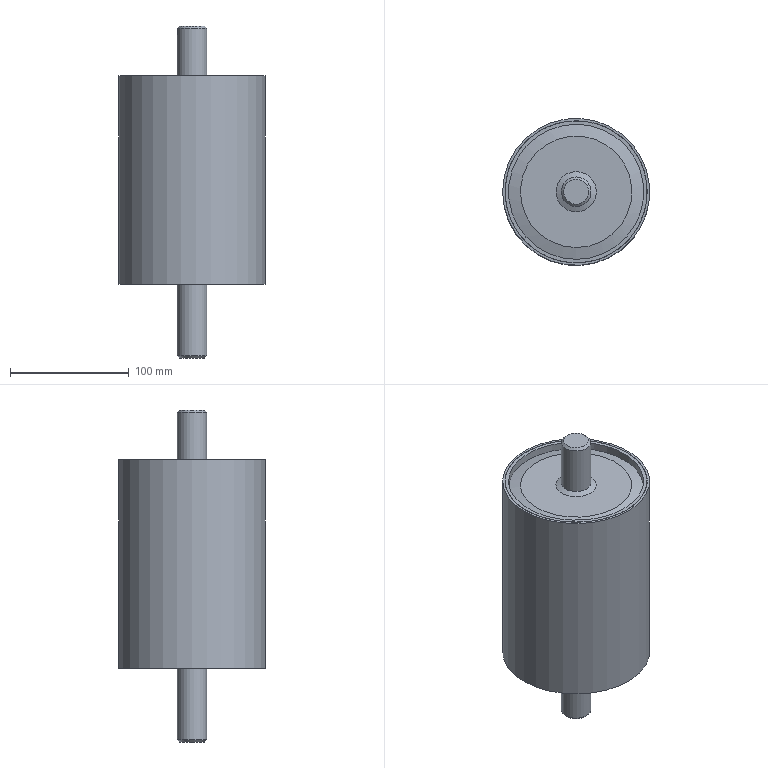Part | STEP file | Pulley | 2 solids | 29 faces | box 124 x 124 x 280 mm | volume 525359 mm3 | cone 10 | plane 10 | cylinder 9 | commonest cylinder face diameters 25 x3 114 x3 120 x2 124 x1
STEP:
#1=CARTESIAN_POINT('',(0.,-10.5,-150.));
#2=VERTEX_POINT('',#1);
#3=CARTESIAN_POINT('',(0.,0.,-150.));
#4=DIRECTION('',(0.,0.,1.));
#5=DIRECTION('',(0.,1.,0.));
#6=AXIS2_PLACEMENT_3D('',#3,#4,#5);
#7=CIRCLE('',#6,10.5);
#8=EDGE_CURVE('',#2,#2,#7,.T.);
#9=ORIENTED_EDGE('',*,*,#8,.T.);
#10=CARTESIAN_POINT('',(0.,-12.5,-148.));
#11=VERTEX_POINT('',#10);
#12=CARTESIAN_POINT('',(0.,-11.5,-149.));
#13=DIRECTION('',(0.,-0.7071,0.7071));
#14=VECTOR('',#13,11.5);
#15=LINE('',#12,#14);
#16=EDGE_CURVE('',#2,#11,#15,.T.);
#17=ORIENTED_EDGE('',*,*,#16,.T.);
#18=CARTESIAN_POINT('',(0.,0.,-148.));
#19=DIRECTION('',(0.,0.,-1.));
#20=DIRECTION('',(0.,1.,0.));
#21=AXIS2_PLACEMENT_3D('',#18,#19,#20);
#22=CIRCLE('',#21,12.5);
#23=EDGE_CURVE('',#11,#11,#22,.T.);
#24=ORIENTED_EDGE('',*,*,#23,.T.);
#25=ORIENTED_EDGE('',*,*,#16,.F.);
#26=EDGE_LOOP('',(#9,#17,#24,#25));
#27=FACE_OUTER_BOUND('',#26,.T.);
#28=CARTESIAN_POINT('',(0.,0.,-149.));
#29=DIRECTION('',(0.,0.,1.));
#30=DIRECTION('',(0.,1.,0.));
#31=AXIS2_PLACEMENT_3D('',#28,#29,#30);
#32=CONICAL_SURFACE('',#31,11.5,0.7854);
#33=ADVANCED_FACE('',(#27),#32,.T.);
#34=ORIENTED_EDGE('',*,*,#8,.F.);
#35=EDGE_LOOP('',(#34));
#36=FACE_OUTER_BOUND('',#35,.T.);
#37=CARTESIAN_POINT('',(0.,0.,-150.));
#38=DIRECTION('',(0.,0.,-1.));
#39=DIRECTION('',(-1.,0.,0.));
#40=AXIS2_PLACEMENT_3D('',#37,#38,#39);
#41=PLANE('',#40);
#42=ADVANCED_FACE('',(#36),#41,.T.);
#43=ORIENTED_EDGE('',*,*,#23,.F.);
#44=CARTESIAN_POINT('',(0.,-12.5,-86.098));
#45=VERTEX_POINT('',#44);
#46=CARTESIAN_POINT('',(0.,-12.5,-108.049));
#47=DIRECTION('',(0.,0.,1.));
#48=VECTOR('',#47,12.5);
#49=LINE('',#46,#48);
#50=EDGE_CURVE('',#11,#45,#49,.T.);
#51=ORIENTED_EDGE('',*,*,#50,.T.);
#52=CARTESIAN_POINT('',(0.,0.,-86.098));
#53=DIRECTION('',(0.,0.,-1.));
#54=DIRECTION('',(1.,0.,0.));
#55=AXIS2_PLACEMENT_3D('',#52,#53,#54);
#56=CIRCLE('',#55,12.5);
#57=EDGE_CURVE('',#45,#45,#56,.T.);
#58=ORIENTED_EDGE('',*,*,#57,.T.);
#59=ORIENTED_EDGE('',*,*,#50,.F.);
#60=EDGE_LOOP('',(#43,#51,#58,#59));
#61=FACE_OUTER_BOUND('',#60,.T.);
#62=CARTESIAN_POINT('',(0.,0.,-108.049));
#63=DIRECTION('',(0.,0.,-1.));
#64=DIRECTION('',(0.,1.,0.));
#65=AXIS2_PLACEMENT_3D('',#62,#63,#64);
#66=CYLINDRICAL_SURFACE('',#65,12.5);
#67=ADVANCED_FACE('',(#61),#66,.T.);
#68=CARTESIAN_POINT('',(0.,12.5,128.));
#69=VERTEX_POINT('',#68);
#70=CARTESIAN_POINT('',(0.,-12.5,128.));
#71=VERTEX_POINT('',#70);
#72=CARTESIAN_POINT('',(0.,0.,128.));
#73=DIRECTION('',(0.,0.,1.));
#74=DIRECTION('',(0.,-1.,0.));
#75=AXIS2_PLACEMENT_3D('',#72,#73,#74);
#76=CIRCLE('',#75,12.5);
#77=EDGE_CURVE('',#69,#71,#76,.T.);
#78=ORIENTED_EDGE('',*,*,#77,.T.);
#79=CARTESIAN_POINT('',(0.,0.,128.));
#80=DIRECTION('',(0.,0.,1.));
#81=DIRECTION('',(0.,-1.,0.));
#82=AXIS2_PLACEMENT_3D('',#79,#80,#81);
#83=CIRCLE('',#82,12.5);
#84=EDGE_CURVE('',#71,#69,#83,.T.);
#85=ORIENTED_EDGE('',*,*,#84,.T.);
#86=CARTESIAN_POINT('',(0.,10.5,130.));
#87=VERTEX_POINT('',#86);
#88=CARTESIAN_POINT('',(0.,11.5,129.));
#89=DIRECTION('',(0.,-0.7071,0.7071));
#90=VECTOR('',#89,11.5);
#91=LINE('',#88,#90);
#92=EDGE_CURVE('',#69,#87,#91,.T.);
#93=ORIENTED_EDGE('',*,*,#92,.T.);
#94=CARTESIAN_POINT('',(0.,0.,130.));
#95=DIRECTION('',(0.,0.,-1.));
#96=DIRECTION('',(0.,-1.,0.));
#97=AXIS2_PLACEMENT_3D('',#94,#95,#96);
#98=CIRCLE('',#97,10.5);
#99=EDGE_CURVE('',#87,#87,#98,.T.);
#100=ORIENTED_EDGE('',*,*,#99,.T.);
#101=ORIENTED_EDGE('',*,*,#92,.F.);
#102=EDGE_LOOP('',(#78,#85,#93,#100,#101));
#103=FACE_OUTER_BOUND('',#102,.T.);
#104=CARTESIAN_POINT('',(0.,0.,129.));
#105=DIRECTION('',(0.,0.,-1.));
#106=DIRECTION('',(0.,-1.,0.));
#107=AXIS2_PLACEMENT_3D('',#104,#105,#106);
#108=CONICAL_SURFACE('',#107,11.5,0.7854);
#109=ADVANCED_FACE('',(#103),#108,.T.);
#110=ORIENTED_EDGE('',*,*,#99,.F.);
#111=EDGE_LOOP('',(#110));
#112=FACE_OUTER_BOUND('',#111,.T.);
#113=CARTESIAN_POINT('',(0.,12.5,130.));
#114=DIRECTION('',(0.,0.,1.));
#115=DIRECTION('',(1.,0.,0.));
#116=AXIS2_PLACEMENT_3D('',#113,#114,#115);
#117=PLANE('',#116);
#118=ADVANCED_FACE('',(#112),#117,.T.);
#119=CARTESIAN_POINT('',(0.,-12.5,86.098));
#120=VERTEX_POINT('',#119);
#121=CARTESIAN_POINT('',(0.,0.,86.098));
#122=DIRECTION('',(0.,0.,-1.));
#123=DIRECTION('',(1.,0.,0.));
#124=AXIS2_PLACEMENT_3D('',#121,#122,#123);
#125=CIRCLE('',#124,12.5);
#126=EDGE_CURVE('',#120,#120,#125,.T.);
#127=ORIENTED_EDGE('',*,*,#126,.F.);
#128=CARTESIAN_POINT('',(0.,-12.5,108.049));
#129=DIRECTION('',(0.,0.,1.));
#130=VECTOR('',#129,12.5);
#131=LINE('',#128,#130);
#132=EDGE_CURVE('',#120,#71,#131,.T.);
#133=ORIENTED_EDGE('',*,*,#132,.T.);
#134=ORIENTED_EDGE('',*,*,#77,.F.);
#135=ORIENTED_EDGE('',*,*,#84,.F.);
#136=ORIENTED_EDGE('',*,*,#132,.F.);
#137=EDGE_LOOP('',(#127,#133,#134,#135,#136));
#138=FACE_OUTER_BOUND('',#137,.T.);
#139=CARTESIAN_POINT('',(0.,0.,108.049));
#140=DIRECTION('',(0.,0.,-1.));
#141=DIRECTION('',(0.,1.,0.));
#142=AXIS2_PLACEMENT_3D('',#139,#140,#141);
#143=CYLINDRICAL_SURFACE('',#142,12.5);
#144=ADVANCED_FACE('',(#138),#143,.T.);
#145=CARTESIAN_POINT('',(0.,-17.,84.));
#146=VERTEX_POINT('',#145);
#147=CARTESIAN_POINT('',(0.,0.,84.));
#148=DIRECTION('',(0.,0.,-1.));
#149=DIRECTION('',(1.,0.,0.));
#150=AXIS2_PLACEMENT_3D('',#147,#148,#149);
#151=CIRCLE('',#150,17.);
#152=EDGE_CURVE('',#146,#146,#151,.T.);
#153=ORIENTED_EDGE('',*,*,#152,.F.);
#154=CARTESIAN_POINT('',(0.,-14.75,85.049));
#155=DIRECTION('',(0.,0.9063,0.4226));
#156=VECTOR('',#155,14.75);
#157=LINE('',#154,#156);
#158=EDGE_CURVE('',#146,#120,#157,.T.);
#159=ORIENTED_EDGE('',*,*,#158,.T.);
#160=ORIENTED_EDGE('',*,*,#126,.T.);
#161=ORIENTED_EDGE('',*,*,#158,.F.);
#162=EDGE_LOOP('',(#153,#159,#160,#161));
#163=FACE_OUTER_BOUND('',#162,.T.);
#164=CARTESIAN_POINT('',(0.,0.,85.049));
#165=DIRECTION('',(0.,0.,-1.));
#166=DIRECTION('',(0.,1.,0.));
#167=AXIS2_PLACEMENT_3D('',#164,#165,#166);
#168=CONICAL_SURFACE('',#167,14.75,1.134);
#169=ADVANCED_FACE('',(#163),#168,.T.);
#170=CARTESIAN_POINT('',(0.,-47.,84.));
#171=VERTEX_POINT('',#170);
#172=CARTESIAN_POINT('',(0.,0.,84.));
#173=DIRECTION('',(0.,0.,-1.));
#174=DIRECTION('',(1.,0.,0.));
#175=AXIS2_PLACEMENT_3D('',#172,#173,#174);
#176=CIRCLE('',#175,47.);
#177=EDGE_CURVE('',#171,#171,#176,.T.);
#178=ORIENTED_EDGE('',*,*,#177,.F.);
#179=EDGE_LOOP('',(#178));
#180=FACE_OUTER_BOUND('',#179,.T.);
#181=ORIENTED_EDGE('',*,*,#152,.T.);
#182=EDGE_LOOP('',(#181));
#183=FACE_BOUND('',#182,.T.);
#184=CARTESIAN_POINT('',(0.,47.,84.));
#185=DIRECTION('',(0.,0.,1.));
#186=DIRECTION('',(1.,0.,0.));
#187=AXIS2_PLACEMENT_3D('',#184,#185,#186);
#188=PLANE('',#187);
#189=ADVANCED_FACE('',(#180,#183),#188,.T.);
#190=CARTESIAN_POINT('',(0.,-57.,81.321));
#191=VERTEX_POINT('',#190);
#192=CARTESIAN_POINT('',(0.,0.,81.321));
#193=DIRECTION('',(0.,0.,-1.));
#194=DIRECTION('',(1.,0.,0.));
#195=AXIS2_PLACEMENT_3D('',#192,#193,#194);
#196=CIRCLE('',#195,57.);
#197=EDGE_CURVE('',#191,#191,#196,.T.);
#198=ORIENTED_EDGE('',*,*,#197,.F.);
#199=CARTESIAN_POINT('',(0.,-52.,82.66));
#200=DIRECTION('',(0.,0.9659,0.2588));
#201=VECTOR('',#200,52.);
#202=LINE('',#199,#201);
#203=EDGE_CURVE('',#191,#171,#202,.T.);
#204=ORIENTED_EDGE('',*,*,#203,.T.);
#205=ORIENTED_EDGE('',*,*,#177,.T.);
#206=ORIENTED_EDGE('',*,*,#203,.F.);
#207=EDGE_LOOP('',(#198,#204,#205,#206));
#208=FACE_OUTER_BOUND('',#207,.T.);
#209=CARTESIAN_POINT('',(0.,0.,82.66));
#210=DIRECTION('',(0.,0.,-1.));
#211=DIRECTION('',(0.,1.,0.));
#212=AXIS2_PLACEMENT_3D('',#209,#210,#211);
#213=CONICAL_SURFACE('',#212,52.,1.309);
#214=ADVANCED_FACE('',(#208),#213,.T.);
#215=ORIENTED_EDGE('',*,*,#197,.T.);
#216=CARTESIAN_POINT('',(0.,-57.,88.));
#217=VERTEX_POINT('',#216);
#218=CARTESIAN_POINT('',(0.,-57.,84.66));
#219=DIRECTION('',(0.,0.,1.));
#220=VECTOR('',#219,57.);
#221=LINE('',#218,#220);
#222=EDGE_CURVE('',#191,#217,#221,.T.);
#223=ORIENTED_EDGE('',*,*,#222,.T.);
#224=CARTESIAN_POINT('',(0.,0.,88.));
#225=DIRECTION('',(0.,0.,-1.));
#226=DIRECTION('',(1.,0.,0.));
#227=AXIS2_PLACEMENT_3D('',#224,#225,#226);
#228=CIRCLE('',#227,57.);
#229=EDGE_CURVE('',#217,#217,#228,.T.);
#230=ORIENTED_EDGE('',*,*,#229,.F.);
#231=ORIENTED_EDGE('',*,*,#222,.F.);
#232=EDGE_LOOP('',(#215,#223,#230,#231));
#233=FACE_OUTER_BOUND('',#232,.T.);
#234=CARTESIAN_POINT('',(0.,0.,84.66));
#235=DIRECTION('',(0.,0.,-1.));
#236=DIRECTION('',(0.,1.,0.));
#237=AXIS2_PLACEMENT_3D('',#234,#235,#236);
#238=CYLINDRICAL_SURFACE('',#237,57.);
#239=ADVANCED_FACE('',(#233),#238,.F.);
#240=CARTESIAN_POINT('',(0.,-60.,88.));
#241=VERTEX_POINT('',#240);
#242=CARTESIAN_POINT('',(0.,0.,88.));
#243=DIRECTION('',(0.,0.,-1.));
#244=DIRECTION('',(1.,0.,0.));
#245=AXIS2_PLACEMENT_3D('',#242,#243,#244);
#246=CIRCLE('',#245,60.);
#247=EDGE_CURVE('',#241,#241,#246,.T.);
#248=ORIENTED_EDGE('',*,*,#247,.F.);
#249=EDGE_LOOP('',(#248));
#250=FACE_OUTER_BOUND('',#249,.T.);
#251=ORIENTED_EDGE('',*,*,#229,.T.);
#252=EDGE_LOOP('',(#251));
#253=FACE_BOUND('',#252,.T.);
#254=CARTESIAN_POINT('',(0.,60.,88.));
#255=DIRECTION('',(0.,0.,1.));
#256=DIRECTION('',(1.,0.,0.));
#257=AXIS2_PLACEMENT_3D('',#254,#255,#256);
#258=PLANE('',#257);
#259=ADVANCED_FACE('',(#250,#253),#258,.T.);
#260=CARTESIAN_POINT('',(0.,-60.,-88.));
#261=VERTEX_POINT('',#260);
#262=CARTESIAN_POINT('',(0.,0.,-88.));
#263=DIRECTION('',(0.,0.,-1.));
#264=DIRECTION('',(1.,0.,0.));
#265=AXIS2_PLACEMENT_3D('',#262,#263,#264);
#266=CIRCLE('',#265,60.);
#267=EDGE_CURVE('',#261,#261,#266,.T.);
#268=ORIENTED_EDGE('',*,*,#267,.F.);
#269=CARTESIAN_POINT('',(0.,-60.,0.));
#270=DIRECTION('',(0.,0.,1.));
#271=VECTOR('',#270,60.);
#272=LINE('',#269,#271);
#273=EDGE_CURVE('',#261,#241,#272,.T.);
#274=ORIENTED_EDGE('',*,*,#273,.T.);
#275=ORIENTED_EDGE('',*,*,#247,.T.);
#276=ORIENTED_EDGE('',*,*,#273,.F.);
#277=EDGE_LOOP('',(#268,#274,#275,#276));
#278=FACE_OUTER_BOUND('',#277,.T.);
#279=CARTESIAN_POINT('',(0.,0.,0.));
#280=DIRECTION('',(0.,0.,-1.));
#281=DIRECTION('',(0.,1.,0.));
#282=AXIS2_PLACEMENT_3D('',#279,#280,#281);
#283=CYLINDRICAL_SURFACE('',#282,60.);
#284=ADVANCED_FACE('',(#278),#283,.T.);
#285=ORIENTED_EDGE('',*,*,#267,.T.);
#286=EDGE_LOOP('',(#285));
#287=FACE_OUTER_BOUND('',#286,.T.);
#288=CARTESIAN_POINT('',(0.,-57.,-88.));
#289=VERTEX_POINT('',#288);
#290=CARTESIAN_POINT('',(0.,0.,-88.));
#291=DIRECTION('',(0.,0.,-1.));
#292=DIRECTION('',(1.,0.,0.));
#293=AXIS2_PLACEMENT_3D('',#290,#291,#292);
#294=CIRCLE('',#293,57.);
#295=EDGE_CURVE('',#289,#289,#294,.T.);
#296=ORIENTED_EDGE('',*,*,#295,.F.);
#297=EDGE_LOOP('',(#296));
#298=FACE_BOUND('',#297,.T.);
#299=CARTESIAN_POINT('',(0.,57.,-88.));
#300=DIRECTION('',(0.,0.,-1.));
#301=DIRECTION('',(-1.,0.,0.));
#302=AXIS2_PLACEMENT_3D('',#299,#300,#301);
#303=PLANE('',#302);
#304=ADVANCED_FACE('',(#287,#298),#303,.T.);
#305=ORIENTED_EDGE('',*,*,#295,.T.);
#306=CARTESIAN_POINT('',(0.,-57.,-81.321));
#307=VERTEX_POINT('',#306);
#308=CARTESIAN_POINT('',(0.,-57.,-84.66));
#309=DIRECTION('',(0.,0.,1.));
#310=VECTOR('',#309,57.);
#311=LINE('',#308,#310);
#312=EDGE_CURVE('',#289,#307,#311,.T.);
#313=ORIENTED_EDGE('',*,*,#312,.T.);
#314=CARTESIAN_POINT('',(0.,0.,-81.321));
#315=DIRECTION('',(0.,0.,-1.));
#316=DIRECTION('',(1.,0.,0.));
#317=AXIS2_PLACEMENT_3D('',#314,#315,#316);
#318=CIRCLE('',#317,57.);
#319=EDGE_CURVE('',#307,#307,#318,.T.);
#320=ORIENTED_EDGE('',*,*,#319,.F.);
#321=ORIENTED_EDGE('',*,*,#312,.F.);
#322=EDGE_LOOP('',(#305,#313,#320,#321));
#323=FACE_OUTER_BOUND('',#322,.T.);
#324=CARTESIAN_POINT('',(0.,0.,-84.66));
#325=DIRECTION('',(0.,0.,-1.));
#326=DIRECTION('',(0.,1.,0.));
#327=AXIS2_PLACEMENT_3D('',#324,#325,#326);
#328=CYLINDRICAL_SURFACE('',#327,57.);
#329=ADVANCED_FACE('',(#323),#328,.F.);
#330=CARTESIAN_POINT('',(0.,-47.,-84.));
#331=VERTEX_POINT('',#330);
#332=CARTESIAN_POINT('',(0.,0.,-84.));
#333=DIRECTION('',(0.,0.,-1.));
#334=DIRECTION('',(1.,0.,0.));
#335=AXIS2_PLACEMENT_3D('',#332,#333,#334);
#336=CIRCLE('',#335,47.);
#337=EDGE_CURVE('',#331,#331,#336,.T.);
#338=ORIENTED_EDGE('',*,*,#337,.F.);
#339=CARTESIAN_POINT('',(0.,-52.,-82.66));
#340=DIRECTION('',(0.,-0.9659,0.2588));
#341=VECTOR('',#340,52.);
#342=LINE('',#339,#341);
#343=EDGE_CURVE('',#331,#307,#342,.T.);
#344=ORIENTED_EDGE('',*,*,#343,.T.);
#345=ORIENTED_EDGE('',*,*,#319,.T.);
#346=ORIENTED_EDGE('',*,*,#343,.F.);
#347=EDGE_LOOP('',(#338,#344,#345,#346));
#348=FACE_OUTER_BOUND('',#347,.T.);
#349=CARTESIAN_POINT('',(0.,0.,-82.66));
#350=DIRECTION('',(0.,0.,1.));
#351=DIRECTION('',(0.,1.,0.));
#352=AXIS2_PLACEMENT_3D('',#349,#350,#351);
#353=CONICAL_SURFACE('',#352,52.,1.309);
#354=ADVANCED_FACE('',(#348),#353,.T.);
#355=ORIENTED_EDGE('',*,*,#337,.T.);
#356=EDGE_LOOP('',(#355));
#357=FACE_OUTER_BOUND('',#356,.T.);
#358=CARTESIAN_POINT('',(0.,-17.,-84.));
#359=VERTEX_POINT('',#358);
#360=CARTESIAN_POINT('',(0.,0.,-84.));
#361=DIRECTION('',(0.,0.,-1.));
#362=DIRECTION('',(1.,0.,0.));
#363=AXIS2_PLACEMENT_3D('',#360,#361,#362);
#364=CIRCLE('',#363,17.);
#365=EDGE_CURVE('',#359,#359,#364,.T.);
#366=ORIENTED_EDGE('',*,*,#365,.F.);
#367=EDGE_LOOP('',(#366));
#368=FACE_BOUND('',#367,.T.);
#369=CARTESIAN_POINT('',(0.,17.,-84.));
#370=DIRECTION('',(0.,0.,-1.));
#371=DIRECTION('',(-1.,0.,0.));
#372=AXIS2_PLACEMENT_3D('',#369,#370,#371);
#373=PLANE('',#372);
#374=ADVANCED_FACE('',(#357,#368),#373,.T.);
#375=ORIENTED_EDGE('',*,*,#57,.F.);
#376=CARTESIAN_POINT('',(0.,-14.75,-85.049));
#377=DIRECTION('',(0.,-0.9063,0.4226));
#378=VECTOR('',#377,14.75);
#379=LINE('',#376,#378);
#380=EDGE_CURVE('',#45,#359,#379,.T.);
#381=ORIENTED_EDGE('',*,*,#380,.T.);
#382=ORIENTED_EDGE('',*,*,#365,.T.);
#383=ORIENTED_EDGE('',*,*,#380,.F.);
#384=EDGE_LOOP('',(#375,#381,#382,#383));
#385=FACE_OUTER_BOUND('',#384,.T.);
#386=CARTESIAN_POINT('',(0.,0.,-85.049));
#387=DIRECTION('',(0.,0.,1.));
#388=DIRECTION('',(0.,1.,0.));
#389=AXIS2_PLACEMENT_3D('',#386,#387,#388);
#390=CONICAL_SURFACE('',#389,14.75,1.134);
#391=ADVANCED_FACE('',(#385),#390,.T.);
#392=CLOSED_SHELL('',(#33,#42,#67,#109,#118,#144,#169,#189,#214,#239,#259,#284,#304,#329,#354,#374,#391));
#393=CARTESIAN_POINT('',(0.,-12.5,-82.792));
#394=VERTEX_POINT('',#393);
#395=CARTESIAN_POINT('',(0.,0.,-82.792));
#396=DIRECTION('',(0.,0.,-1.));
#397=DIRECTION('',(1.,0.,0.));
#398=AXIS2_PLACEMENT_3D('',#395,#396,#397);
#399=CIRCLE('',#398,12.5);
#400=EDGE_CURVE('',#394,#394,#399,.T.);
#401=ORIENTED_EDGE('',*,*,#400,.T.);
#402=CARTESIAN_POINT('',(0.,-16.335,-81.));
#403=VERTEX_POINT('',#402);
#404=CARTESIAN_POINT('',(0.,-14.417,-81.896));
#405=DIRECTION('',(0.,-0.906,0.4233));
#406=VECTOR('',#405,14.417);
#407=LINE('',#404,#406);
#408=EDGE_CURVE('',#394,#403,#407,.T.);
#409=ORIENTED_EDGE('',*,*,#408,.T.);
#410=CARTESIAN_POINT('',(0.,0.,-81.));
#411=DIRECTION('',(0.,0.,-1.));
#412=DIRECTION('',(1.,0.,0.));
#413=AXIS2_PLACEMENT_3D('',#410,#411,#412);
#414=CIRCLE('',#413,16.335);
#415=EDGE_CURVE('',#403,#403,#414,.T.);
#416=ORIENTED_EDGE('',*,*,#415,.F.);
#417=ORIENTED_EDGE('',*,*,#408,.F.);
#418=EDGE_LOOP('',(#401,#409,#416,#417));
#419=FACE_OUTER_BOUND('',#418,.T.);
#420=CARTESIAN_POINT('',(0.,0.,-81.896));
#421=DIRECTION('',(0.,0.,1.));
#422=DIRECTION('',(0.,1.,0.));
#423=AXIS2_PLACEMENT_3D('',#420,#421,#422);
#424=CONICAL_SURFACE('',#423,14.417,1.134);
#425=ADVANCED_FACE('',(#419),#424,.F.);
#426=ORIENTED_EDGE('',*,*,#400,.F.);
#427=CARTESIAN_POINT('',(0.,-12.5,82.792));
#428=VERTEX_POINT('',#427);
#429=CARTESIAN_POINT('',(0.,-12.5,0.));
#430=DIRECTION('',(0.,0.,1.));
#431=VECTOR('',#430,12.5);
#432=LINE('',#429,#431);
#433=EDGE_CURVE('',#394,#428,#432,.T.);
#434=ORIENTED_EDGE('',*,*,#433,.T.);
#435=CARTESIAN_POINT('',(0.,0.,82.792));
#436=DIRECTION('',(0.,0.,-1.));
#437=DIRECTION('',(1.,0.,0.));
#438=AXIS2_PLACEMENT_3D('',#435,#436,#437);
#439=CIRCLE('',#438,12.5);
#440=EDGE_CURVE('',#428,#428,#439,.T.);
#441=ORIENTED_EDGE('',*,*,#440,.T.);
#442=ORIENTED_EDGE('',*,*,#433,.F.);
#443=EDGE_LOOP('',(#426,#434,#441,#442));
#444=FACE_OUTER_BOUND('',#443,.T.);
#445=CARTESIAN_POINT('',(0.,0.,0.));
#446=DIRECTION('',(0.,0.,-1.));
#447=DIRECTION('',(0.,1.,0.));
#448=AXIS2_PLACEMENT_3D('',#445,#446,#447);
#449=CYLINDRICAL_SURFACE('',#448,12.5);
#450=ADVANCED_FACE('',(#444),#449,.T.);
#451=CARTESIAN_POINT('',(0.,-46.605,-81.));
#452=VERTEX_POINT('',#451);
#453=CARTESIAN_POINT('',(0.,0.,-81.));
#454=DIRECTION('',(0.,0.,-1.));
#455=DIRECTION('',(1.,0.,0.));
#456=AXIS2_PLACEMENT_3D('',#453,#454,#455);
#457=CIRCLE('',#456,46.605);
#458=EDGE_CURVE('',#452,#452,#457,.T.);
#459=ORIENTED_EDGE('',*,*,#458,.F.);
#460=EDGE_LOOP('',(#459));
#461=FACE_OUTER_BOUND('',#460,.T.);
#462=ORIENTED_EDGE('',*,*,#415,.T.);
#463=EDGE_LOOP('',(#462));
#464=FACE_BOUND('',#463,.T.);
#465=CARTESIAN_POINT('',(0.,46.605,-81.));
#466=DIRECTION('',(0.,0.,1.));
#467=DIRECTION('',(1.,0.,0.));
#468=AXIS2_PLACEMENT_3D('',#465,#466,#467);
#469=PLANE('',#468);
#470=ADVANCED_FACE('',(#461,#464),#469,.T.);
#471=CARTESIAN_POINT('',(0.,-16.335,81.));
#472=VERTEX_POINT('',#471);
#473=CARTESIAN_POINT('',(0.,0.,81.));
#474=DIRECTION('',(0.,0.,-1.));
#475=DIRECTION('',(1.,0.,0.));
#476=AXIS2_PLACEMENT_3D('',#473,#474,#475);
#477=CIRCLE('',#476,16.335);
#478=EDGE_CURVE('',#472,#472,#477,.T.);
#479=ORIENTED_EDGE('',*,*,#478,.T.);
#480=CARTESIAN_POINT('',(0.,-14.417,81.896));
#481=DIRECTION('',(0.,0.906,0.4233));
#482=VECTOR('',#481,14.417);
#483=LINE('',#480,#482);
#484=EDGE_CURVE('',#472,#428,#483,.T.);
#485=ORIENTED_EDGE('',*,*,#484,.T.);
#486=ORIENTED_EDGE('',*,*,#440,.F.);
#487=ORIENTED_EDGE('',*,*,#484,.F.);
#488=EDGE_LOOP('',(#479,#485,#486,#487));
#489=FACE_OUTER_BOUND('',#488,.T.);
#490=CARTESIAN_POINT('',(0.,0.,81.896));
#491=DIRECTION('',(0.,0.,-1.));
#492=DIRECTION('',(0.,1.,0.));
#493=AXIS2_PLACEMENT_3D('',#490,#491,#492);
#494=CONICAL_SURFACE('',#493,14.417,1.134);
#495=ADVANCED_FACE('',(#489),#494,.F.);
#496=ORIENTED_EDGE('',*,*,#458,.T.);
#497=CARTESIAN_POINT('',(0.,-57.,-78.218));
#498=VERTEX_POINT('',#497);
#499=CARTESIAN_POINT('',(0.,-51.803,-79.609));
#500=DIRECTION('',(0.,-0.966,0.2585));
#501=VECTOR('',#500,51.803);
#502=LINE('',#499,#501);
#503=EDGE_CURVE('',#452,#498,#502,.T.);
#504=ORIENTED_EDGE('',*,*,#503,.T.);
#505=CARTESIAN_POINT('',(0.,0.,-78.218));
#506=DIRECTION('',(0.,0.,-1.));
#507=DIRECTION('',(1.,0.,0.));
#508=AXIS2_PLACEMENT_3D('',#505,#506,#507);
#509=CIRCLE('',#508,57.);
#510=EDGE_CURVE('',#498,#498,#509,.T.);
#511=ORIENTED_EDGE('',*,*,#510,.F.);
#512=ORIENTED_EDGE('',*,*,#503,.F.);
#513=EDGE_LOOP('',(#496,#504,#511,#512));
#514=FACE_OUTER_BOUND('',#513,.T.);
#515=CARTESIAN_POINT('',(0.,0.,-79.609));
#516=DIRECTION('',(0.,0.,1.));
#517=DIRECTION('',(0.,1.,0.));
#518=AXIS2_PLACEMENT_3D('',#515,#516,#517);
#519=CONICAL_SURFACE('',#518,51.803,1.309);
#520=ADVANCED_FACE('',(#514),#519,.F.);
#521=CARTESIAN_POINT('',(0.,-46.605,81.));
#522=VERTEX_POINT('',#521);
#523=CARTESIAN_POINT('',(0.,0.,81.));
#524=DIRECTION('',(0.,0.,-1.));
#525=DIRECTION('',(1.,0.,0.));
#526=AXIS2_PLACEMENT_3D('',#523,#524,#525);
#527=CIRCLE('',#526,46.605);
#528=EDGE_CURVE('',#522,#522,#527,.T.);
#529=ORIENTED_EDGE('',*,*,#528,.T.);
#530=EDGE_LOOP('',(#529));
#531=FACE_OUTER_BOUND('',#530,.T.);
#532=ORIENTED_EDGE('',*,*,#478,.F.);
#533=EDGE_LOOP('',(#532));
#534=FACE_BOUND('',#533,.T.);
#535=CARTESIAN_POINT('',(0.,16.335,81.));
#536=DIRECTION('',(0.,0.,-1.));
#537=DIRECTION('',(-1.,0.,0.));
#538=AXIS2_PLACEMENT_3D('',#535,#536,#537);
#539=PLANE('',#538);
#540=ADVANCED_FACE('',(#531,#534),#539,.T.);
#541=ORIENTED_EDGE('',*,*,#510,.T.);
#542=CARTESIAN_POINT('',(0.,-57.,78.218));
#543=VERTEX_POINT('',#542);
#544=CARTESIAN_POINT('',(0.,-57.,0.));
#545=DIRECTION('',(0.,0.,1.));
#546=VECTOR('',#545,57.);
#547=LINE('',#544,#546);
#548=EDGE_CURVE('',#498,#543,#547,.T.);
#549=ORIENTED_EDGE('',*,*,#548,.T.);
#550=CARTESIAN_POINT('',(0.,0.,78.218));
#551=DIRECTION('',(0.,0.,-1.));
#552=DIRECTION('',(1.,0.,0.));
#553=AXIS2_PLACEMENT_3D('',#550,#551,#552);
#554=CIRCLE('',#553,57.);
#555=EDGE_CURVE('',#543,#543,#554,.T.);
#556=ORIENTED_EDGE('',*,*,#555,.F.);
#557=ORIENTED_EDGE('',*,*,#548,.F.);
#558=EDGE_LOOP('',(#541,#549,#556,#557));
#559=FACE_OUTER_BOUND('',#558,.T.);
#560=CARTESIAN_POINT('',(0.,0.,0.));
#561=DIRECTION('',(0.,0.,-1.));
#562=DIRECTION('',(0.,1.,0.));
#563=AXIS2_PLACEMENT_3D('',#560,#561,#562);
#564=CYLINDRICAL_SURFACE('',#563,57.);
#565=ADVANCED_FACE('',(#559),#564,.F.);
#566=ORIENTED_EDGE('',*,*,#555,.T.);
#567=CARTESIAN_POINT('',(0.,-51.803,79.609));
#568=DIRECTION('',(0.,0.966,0.2585));
#569=VECTOR('',#568,51.803);
#570=LINE('',#567,#569);
#571=EDGE_CURVE('',#543,#522,#570,.T.);
#572=ORIENTED_EDGE('',*,*,#571,.T.);
#573=ORIENTED_EDGE('',*,*,#528,.F.);
#574=ORIENTED_EDGE('',*,*,#571,.F.);
#575=EDGE_LOOP('',(#566,#572,#573,#574));
#576=FACE_OUTER_BOUND('',#575,.T.);
#577=CARTESIAN_POINT('',(0.,0.,79.609));
#578=DIRECTION('',(0.,0.,-1.));
#579=DIRECTION('',(0.,1.,0.));
#580=AXIS2_PLACEMENT_3D('',#577,#578,#579);
#581=CONICAL_SURFACE('',#580,51.803,1.309);
#582=ADVANCED_FACE('',(#576),#581,.F.);
#583=CLOSED_SHELL('',(#425,#450,#470,#495,#520,#540,#565,#582));
#584=ORIENTED_CLOSED_SHELL('',*,#583,.F.);
#585=BREP_WITH_VOIDS('',#392,(#584));
#586=CARTESIAN_POINT('',(60.,0.,-88.));
#587=VERTEX_POINT('',#586);
#588=CARTESIAN_POINT('',(0.,0.,-88.));
#589=DIRECTION('',(0.,0.,-1.));
#590=DIRECTION('',(-1.,0.,0.));
#591=AXIS2_PLACEMENT_3D('',#588,#589,#590);
#592=CIRCLE('',#591,60.);
#593=EDGE_CURVE('',#587,#587,#592,.T.);
#594=ORIENTED_EDGE('',*,*,#593,.T.);
#595=CARTESIAN_POINT('',(60.,0.,88.));
#596=VERTEX_POINT('',#595);
#597=CARTESIAN_POINT('',(60.,0.,88.));
#598=DIRECTION('',(0.,0.,1.));
#599=VECTOR('',#598,60.);
#600=LINE('',#597,#599);
#601=EDGE_CURVE('',#587,#596,#600,.T.);
#602=ORIENTED_EDGE('',*,*,#601,.T.);
#603=CARTESIAN_POINT('',(0.,0.,88.));
#604=DIRECTION('',(0.,0.,-1.));
#605=DIRECTION('',(-1.,0.,0.));
#606=AXIS2_PLACEMENT_3D('',#603,#604,#605);
#607=CIRCLE('',#606,60.);
#608=EDGE_CURVE('',#596,#596,#607,.T.);
#609=ORIENTED_EDGE('',*,*,#608,.F.);
#610=ORIENTED_EDGE('',*,*,#601,.F.);
#611=EDGE_LOOP('',(#594,#602,#609,#610));
#612=FACE_OUTER_BOUND('',#611,.T.);
#613=CARTESIAN_POINT('',(0.,0.,88.));
#614=DIRECTION('',(0.,0.,-1.));
#615=DIRECTION('',(-1.,0.,0.));
#616=AXIS2_PLACEMENT_3D('',#613,#614,#615);
#617=CYLINDRICAL_SURFACE('',#616,60.);
#618=ADVANCED_FACE('',(#612),#617,.F.);
#619=CARTESIAN_POINT('',(-62.,0.,-88.));
#620=VERTEX_POINT('',#619);
#621=CARTESIAN_POINT('',(0.,0.,-88.));
#622=DIRECTION('',(0.,0.,1.));
#623=DIRECTION('',(1.,0.,0.));
#624=AXIS2_PLACEMENT_3D('',#621,#622,#623);
#625=CIRCLE('',#624,62.);
#626=EDGE_CURVE('',#620,#620,#625,.T.);
#627=ORIENTED_EDGE('',*,*,#626,.T.);
#628=CARTESIAN_POINT('',(-62.,0.,88.));
#629=VERTEX_POINT('',#628);
#630=CARTESIAN_POINT('',(-62.,0.,88.));
#631=DIRECTION('',(0.,0.,1.));
#632=VECTOR('',#631,62.);
#633=LINE('',#630,#632);
#634=EDGE_CURVE('',#620,#629,#633,.T.);
#635=ORIENTED_EDGE('',*,*,#634,.T.);
#636=CARTESIAN_POINT('',(0.,0.,88.));
#637=DIRECTION('',(0.,0.,1.));
#638=DIRECTION('',(1.,0.,0.));
#639=AXIS2_PLACEMENT_3D('',#636,#637,#638);
#640=CIRCLE('',#639,62.);
#641=EDGE_CURVE('',#629,#629,#640,.T.);
#642=ORIENTED_EDGE('',*,*,#641,.F.);
#643=ORIENTED_EDGE('',*,*,#634,.F.);
#644=EDGE_LOOP('',(#627,#635,#642,#643));
#645=FACE_OUTER_BOUND('',#644,.T.);
#646=CARTESIAN_POINT('',(0.,0.,88.));
#647=DIRECTION('',(0.,0.,-1.));
#648=DIRECTION('',(1.,0.,0.));
#649=AXIS2_PLACEMENT_3D('',#646,#647,#648);
#650=CYLINDRICAL_SURFACE('',#649,62.);
#651=ADVANCED_FACE('',(#645),#650,.T.);
#652=ORIENTED_EDGE('',*,*,#641,.T.);
#653=EDGE_LOOP('',(#652));
#654=FACE_OUTER_BOUND('',#653,.T.);
#655=ORIENTED_EDGE('',*,*,#608,.T.);
#656=EDGE_LOOP('',(#655));
#657=FACE_BOUND('',#656,.T.);
#658=CARTESIAN_POINT('',(0.,0.,88.));
#659=DIRECTION('',(0.,0.,1.));
#660=DIRECTION('',(1.,0.,0.));
#661=AXIS2_PLACEMENT_3D('',#658,#659,#660);
#662=PLANE('',#661);
#663=ADVANCED_FACE('',(#654,#657),#662,.T.);
#664=ORIENTED_EDGE('',*,*,#626,.F.);
#665=EDGE_LOOP('',(#664));
#666=FACE_OUTER_BOUND('',#665,.T.);
#667=ORIENTED_EDGE('',*,*,#593,.F.);
#668=EDGE_LOOP('',(#667));
#669=FACE_BOUND('',#668,.T.);
#670=CARTESIAN_POINT('',(0.,0.,-88.));
#671=DIRECTION('',(0.,0.,-1.));
#672=DIRECTION('',(-1.,0.,0.));
#673=AXIS2_PLACEMENT_3D('',#670,#671,#672);
#674=PLANE('',#673);
#675=ADVANCED_FACE('',(#666,#669),#674,.T.);
#676=CLOSED_SHELL('',(#618,#651,#663,#675));
#677=MANIFOLD_SOLID_BREP('',#676);
#678=(LENGTH_UNIT()NAMED_UNIT(*)SI_UNIT(.MILLI.,.METRE.));
#679=UNCERTAINTY_MEASURE_WITH_UNIT(LENGTH_MEASURE(0.01),#678,'','');
#680=(NAMED_UNIT(*)PLANE_ANGLE_UNIT()SI_UNIT($,.RADIAN.));
#681=(NAMED_UNIT(*)SI_UNIT($,.STERADIAN.)SOLID_ANGLE_UNIT());
#682=(GEOMETRIC_REPRESENTATION_CONTEXT(3)GLOBAL_UNCERTAINTY_ASSIGNED_CONTEXT((#679))GLOBAL_UNIT_ASSIGNED_CONTEXT((#678,#680,#681))REPRESENTATION_CONTEXT('',''));
#683=ADVANCED_BREP_SHAPE_REPRESENTATION('',(#585,#677),#682);